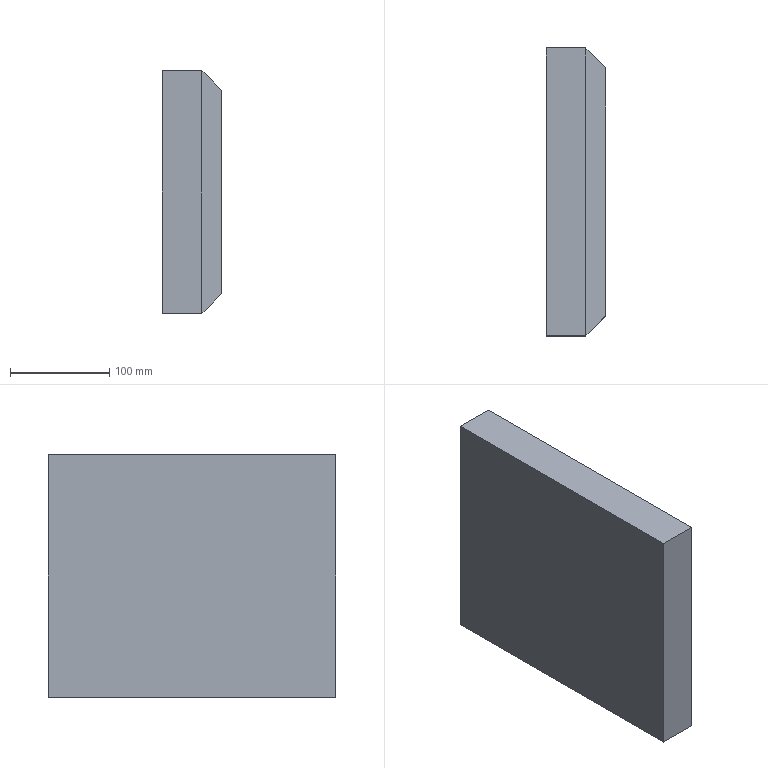Part | SolidWorks | features SplitBody 1 | 1 solid | 10 faces | box 60 x 290 x 245 mm | volume 4059667 mm3 | plane 10
STEP:
#1=CARTESIAN_POINT('',(2951.,873.44,-805.));
#2=VERTEX_POINT('',#1);
#3=CARTESIAN_POINT('',(2951.,583.44,-805.));
#4=VERTEX_POINT('',#3);
#5=CARTESIAN_POINT('',(2951.,583.44,-805.));
#6=DIRECTION('',(0.,-1.,0.));
#7=VECTOR('',#6,1000.);
#8=LINE('',#5,#7);
#9=EDGE_CURVE('',#2,#4,#8,.T.);
#10=ORIENTED_EDGE('',*,*,#9,.F.);
#11=CARTESIAN_POINT('',(2951.,873.44,-1050.));
#12=VERTEX_POINT('',#11);
#13=CARTESIAN_POINT('',(2951.,873.44,-1050.));
#14=DIRECTION('',(0.,0.,1.));
#15=VECTOR('',#14,1000.);
#16=LINE('',#13,#15);
#17=EDGE_CURVE('',#12,#2,#16,.T.);
#18=ORIENTED_EDGE('',*,*,#17,.F.);
#19=CARTESIAN_POINT('',(2951.,583.44,-1050.));
#20=VERTEX_POINT('',#19);
#21=CARTESIAN_POINT('',(2951.,583.44,-1050.));
#22=DIRECTION('',(0.,1.,0.));
#23=VECTOR('',#22,1000.);
#24=LINE('',#21,#23);
#25=EDGE_CURVE('',#20,#12,#24,.T.);
#26=ORIENTED_EDGE('',*,*,#25,.F.);
#27=CARTESIAN_POINT('',(2951.,583.44,-1050.));
#28=DIRECTION('',(0.,0.,-1.));
#29=VECTOR('',#28,1000.);
#30=LINE('',#27,#29);
#31=EDGE_CURVE('',#4,#20,#30,.T.);
#32=ORIENTED_EDGE('',*,*,#31,.F.);
#33=EDGE_LOOP('',(#10,#18,#26,#32));
#34=FACE_OUTER_BOUND('',#33,.T.);
#35=CARTESIAN_POINT('',(2951.,583.44,-1050.));
#36=DIRECTION('',(1.,0.,0.));
#37=DIRECTION('',(0.,1.,0.));
#38=AXIS2_PLACEMENT_3D('',#35,#36,#37);
#39=PLANE('',#38);
#40=ADVANCED_FACE('',(#34),#39,.F.);
#41=CARTESIAN_POINT('',(2991.,583.44,-805.));
#42=VERTEX_POINT('',#41);
#43=CARTESIAN_POINT('',(2991.,583.44,-1050.));
#44=VERTEX_POINT('',#43);
#45=CARTESIAN_POINT('',(2991.,583.44,-805.));
#46=DIRECTION('',(0.,0.,-1.));
#47=VECTOR('',#46,1000.);
#48=LINE('',#45,#47);
#49=EDGE_CURVE('',#42,#44,#48,.T.);
#50=ORIENTED_EDGE('',*,*,#49,.F.);
#51=CARTESIAN_POINT('',(3011.,583.44,-805.));
#52=DIRECTION('',(1.,0.,0.));
#53=VECTOR('',#52,1000.);
#54=LINE('',#51,#53);
#55=EDGE_CURVE('',#4,#42,#54,.T.);
#56=ORIENTED_EDGE('',*,*,#55,.F.);
#57=ORIENTED_EDGE('',*,*,#31,.T.);
#58=CARTESIAN_POINT('',(3011.,583.44,-1050.));
#59=DIRECTION('',(-1.,0.,0.));
#60=VECTOR('',#59,1000.);
#61=LINE('',#58,#60);
#62=EDGE_CURVE('',#44,#20,#61,.T.);
#63=ORIENTED_EDGE('',*,*,#62,.F.);
#64=EDGE_LOOP('',(#50,#56,#57,#63));
#65=FACE_OUTER_BOUND('',#64,.T.);
#66=CARTESIAN_POINT('',(3011.,583.44,-805.));
#67=DIRECTION('',(0.,1.,0.));
#68=DIRECTION('',(0.,0.,1.));
#69=AXIS2_PLACEMENT_3D('',#66,#67,#68);
#70=PLANE('',#69);
#71=ADVANCED_FACE('',(#65),#70,.F.);
#72=CARTESIAN_POINT('',(2991.,873.44,-805.));
#73=VERTEX_POINT('',#72);
#74=CARTESIAN_POINT('',(2991.,583.44,-805.));
#75=DIRECTION('',(0.,-1.,0.));
#76=VECTOR('',#75,1000.);
#77=LINE('',#74,#76);
#78=EDGE_CURVE('',#73,#42,#77,.T.);
#79=ORIENTED_EDGE('',*,*,#78,.F.);
#80=CARTESIAN_POINT('',(3011.,873.44,-805.));
#81=DIRECTION('',(1.,0.,0.));
#82=VECTOR('',#81,1000.);
#83=LINE('',#80,#82);
#84=EDGE_CURVE('',#2,#73,#83,.T.);
#85=ORIENTED_EDGE('',*,*,#84,.F.);
#86=ORIENTED_EDGE('',*,*,#9,.T.);
#87=ORIENTED_EDGE('',*,*,#55,.T.);
#88=EDGE_LOOP('',(#79,#85,#86,#87));
#89=FACE_OUTER_BOUND('',#88,.T.);
#90=CARTESIAN_POINT('',(3011.,583.44,-805.));
#91=DIRECTION('',(0.,0.,-1.));
#92=DIRECTION('',(-1.,0.,0.));
#93=AXIS2_PLACEMENT_3D('',#90,#91,#92);
#94=PLANE('',#93);
#95=ADVANCED_FACE('',(#89),#94,.F.);
#96=CARTESIAN_POINT('',(2991.,873.44,-1050.));
#97=VERTEX_POINT('',#96);
#98=CARTESIAN_POINT('',(2991.,873.44,-805.));
#99=DIRECTION('',(0.,0.,1.));
#100=VECTOR('',#99,1000.);
#101=LINE('',#98,#100);
#102=EDGE_CURVE('',#97,#73,#101,.T.);
#103=ORIENTED_EDGE('',*,*,#102,.F.);
#104=CARTESIAN_POINT('',(3011.,873.44,-1050.));
#105=DIRECTION('',(1.,0.,0.));
#106=VECTOR('',#105,1000.);
#107=LINE('',#104,#106);
#108=EDGE_CURVE('',#12,#97,#107,.T.);
#109=ORIENTED_EDGE('',*,*,#108,.F.);
#110=ORIENTED_EDGE('',*,*,#17,.T.);
#111=ORIENTED_EDGE('',*,*,#84,.T.);
#112=EDGE_LOOP('',(#103,#109,#110,#111));
#113=FACE_OUTER_BOUND('',#112,.T.);
#114=CARTESIAN_POINT('',(3011.,873.44,-805.));
#115=DIRECTION('',(0.,-1.,0.));
#116=DIRECTION('',(0.,0.,-1.));
#117=AXIS2_PLACEMENT_3D('',#114,#115,#116);
#118=PLANE('',#117);
#119=ADVANCED_FACE('',(#113),#118,.F.);
#120=CARTESIAN_POINT('',(2991.,583.44,-1050.));
#121=DIRECTION('',(0.,1.,0.));
#122=VECTOR('',#121,1000.);
#123=LINE('',#120,#122);
#124=EDGE_CURVE('',#44,#97,#123,.T.);
#125=ORIENTED_EDGE('',*,*,#124,.F.);
#126=ORIENTED_EDGE('',*,*,#62,.T.);
#127=ORIENTED_EDGE('',*,*,#25,.T.);
#128=ORIENTED_EDGE('',*,*,#108,.T.);
#129=EDGE_LOOP('',(#125,#126,#127,#128));
#130=FACE_OUTER_BOUND('',#129,.T.);
#131=CARTESIAN_POINT('',(3011.,583.44,-1050.));
#132=DIRECTION('',(0.,0.,1.));
#133=DIRECTION('',(1.,0.,0.));
#134=AXIS2_PLACEMENT_3D('',#131,#132,#133);
#135=PLANE('',#134);
#136=ADVANCED_FACE('',(#130),#135,.F.);
#137=CARTESIAN_POINT('',(3011.,603.44,-825.));
#138=VERTEX_POINT('',#137);
#139=CARTESIAN_POINT('',(3011.,603.44,-825.));
#140=DIRECTION('',(-0.5774,-0.5774,0.5774));
#141=VECTOR('',#140,1000.);
#142=LINE('',#139,#141);
#143=EDGE_CURVE('',#138,#42,#142,.T.);
#144=ORIENTED_EDGE('',*,*,#143,.T.);
#145=ORIENTED_EDGE('',*,*,#49,.T.);
#146=CARTESIAN_POINT('',(3011.,603.44,-1030.));
#147=VERTEX_POINT('',#146);
#148=CARTESIAN_POINT('',(2991.,583.44,-1050.));
#149=DIRECTION('',(0.5774,0.5774,0.5774));
#150=VECTOR('',#149,1000.);
#151=LINE('',#148,#150);
#152=EDGE_CURVE('',#44,#147,#151,.T.);
#153=ORIENTED_EDGE('',*,*,#152,.T.);
#154=CARTESIAN_POINT('',(3011.,603.44,-1050.));
#155=DIRECTION('',(0.,0.,1.));
#156=VECTOR('',#155,1000.);
#157=LINE('',#154,#156);
#158=EDGE_CURVE('',#147,#138,#157,.T.);
#159=ORIENTED_EDGE('',*,*,#158,.T.);
#160=EDGE_LOOP('',(#144,#145,#153,#159));
#161=FACE_OUTER_BOUND('',#160,.T.);
#162=CARTESIAN_POINT('',(3011.,603.44,-1050.));
#163=DIRECTION('',(0.7071,-0.7071,0.));
#164=DIRECTION('',(0.7071,0.7071,0.));
#165=AXIS2_PLACEMENT_3D('',#162,#163,#164);
#166=PLANE('',#165);
#167=ADVANCED_FACE('',(#161),#166,.T.);
#168=ORIENTED_EDGE('',*,*,#143,.F.);
#169=CARTESIAN_POINT('',(3011.,853.44,-825.));
#170=VERTEX_POINT('',#169);
#171=CARTESIAN_POINT('',(3011.,583.44,-825.));
#172=DIRECTION('',(0.,1.,0.));
#173=VECTOR('',#172,1000.);
#174=LINE('',#171,#173);
#175=EDGE_CURVE('',#138,#170,#174,.T.);
#176=ORIENTED_EDGE('',*,*,#175,.T.);
#177=CARTESIAN_POINT('',(3011.,853.44,-825.));
#178=DIRECTION('',(-0.5774,0.5774,0.5774));
#179=VECTOR('',#178,1000.);
#180=LINE('',#177,#179);
#181=EDGE_CURVE('',#170,#73,#180,.T.);
#182=ORIENTED_EDGE('',*,*,#181,.T.);
#183=ORIENTED_EDGE('',*,*,#78,.T.);
#184=EDGE_LOOP('',(#168,#176,#182,#183));
#185=FACE_OUTER_BOUND('',#184,.T.);
#186=CARTESIAN_POINT('',(3011.,583.44,-825.));
#187=DIRECTION('',(0.7071,0.,0.7071));
#188=DIRECTION('',(0.7071,0.,-0.7071));
#189=AXIS2_PLACEMENT_3D('',#186,#187,#188);
#190=PLANE('',#189);
#191=ADVANCED_FACE('',(#185),#190,.T.);
#192=ORIENTED_EDGE('',*,*,#181,.F.);
#193=CARTESIAN_POINT('',(3011.,853.44,-1030.));
#194=VERTEX_POINT('',#193);
#195=CARTESIAN_POINT('',(3011.,853.44,-1050.));
#196=DIRECTION('',(0.,0.,-1.));
#197=VECTOR('',#196,1000.);
#198=LINE('',#195,#197);
#199=EDGE_CURVE('',#170,#194,#198,.T.);
#200=ORIENTED_EDGE('',*,*,#199,.T.);
#201=CARTESIAN_POINT('',(3011.,853.44,-1030.));
#202=DIRECTION('',(-0.5774,0.5774,-0.5774));
#203=VECTOR('',#202,1000.);
#204=LINE('',#201,#203);
#205=EDGE_CURVE('',#194,#97,#204,.T.);
#206=ORIENTED_EDGE('',*,*,#205,.T.);
#207=ORIENTED_EDGE('',*,*,#102,.T.);
#208=EDGE_LOOP('',(#192,#200,#206,#207));
#209=FACE_OUTER_BOUND('',#208,.T.);
#210=CARTESIAN_POINT('',(3011.,853.44,-1050.));
#211=DIRECTION('',(0.7071,0.7071,0.));
#212=DIRECTION('',(-0.7071,0.7071,0.));
#213=AXIS2_PLACEMENT_3D('',#210,#211,#212);
#214=PLANE('',#213);
#215=ADVANCED_FACE('',(#209),#214,.T.);
#216=ORIENTED_EDGE('',*,*,#205,.F.);
#217=CARTESIAN_POINT('',(3011.,583.44,-1030.));
#218=DIRECTION('',(0.,-1.,0.));
#219=VECTOR('',#218,1000.);
#220=LINE('',#217,#219);
#221=EDGE_CURVE('',#194,#147,#220,.T.);
#222=ORIENTED_EDGE('',*,*,#221,.T.);
#223=ORIENTED_EDGE('',*,*,#152,.F.);
#224=ORIENTED_EDGE('',*,*,#124,.T.);
#225=EDGE_LOOP('',(#216,#222,#223,#224));
#226=FACE_OUTER_BOUND('',#225,.T.);
#227=CARTESIAN_POINT('',(3011.,583.44,-1030.));
#228=DIRECTION('',(0.7071,0.,-0.7071));
#229=DIRECTION('',(-0.7071,0.,-0.7071));
#230=AXIS2_PLACEMENT_3D('',#227,#228,#229);
#231=PLANE('',#230);
#232=ADVANCED_FACE('',(#226),#231,.T.);
#233=ORIENTED_EDGE('',*,*,#158,.F.);
#234=ORIENTED_EDGE('',*,*,#221,.F.);
#235=ORIENTED_EDGE('',*,*,#199,.F.);
#236=ORIENTED_EDGE('',*,*,#175,.F.);
#237=EDGE_LOOP('',(#233,#234,#235,#236));
#238=FACE_OUTER_BOUND('',#237,.T.);
#239=CARTESIAN_POINT('',(3011.,583.44,-1050.));
#240=DIRECTION('',(1.,0.,0.));
#241=DIRECTION('',(0.,1.,0.));
#242=AXIS2_PLACEMENT_3D('',#239,#240,#241);
#243=PLANE('',#242);
#244=ADVANCED_FACE('',(#238),#243,.T.);
#245=CLOSED_SHELL('',(#40,#71,#95,#119,#136,#167,#191,#215,#232,#244));
#246=MANIFOLD_SOLID_BREP('',#245);
#247=CARTESIAN_POINT('',(0.,0.,0.));
#248=DIRECTION('',(0.,0.,1.));
#249=DIRECTION('',(1.,0.,0.));
#250=AXIS2_PLACEMENT_3D('',#247,#248,#249);
#251=(LENGTH_UNIT()NAMED_UNIT(*)SI_UNIT(.MILLI.,.METRE.));
#252=UNCERTAINTY_MEASURE_WITH_UNIT(LENGTH_MEASURE(0.00001),#251,'','');
#253=(NAMED_UNIT(*)PLANE_ANGLE_UNIT()SI_UNIT($,.RADIAN.));
#254=(NAMED_UNIT(*)SI_UNIT($,.STERADIAN.)SOLID_ANGLE_UNIT());
#255=(GEOMETRIC_REPRESENTATION_CONTEXT(3)GLOBAL_UNCERTAINTY_ASSIGNED_CONTEXT((#252))GLOBAL_UNIT_ASSIGNED_CONTEXT((#251,#253,#254))REPRESENTATION_CONTEXT('',''));
#256=ADVANCED_BREP_SHAPE_REPRESENTATION('',(#246,#250),#255);